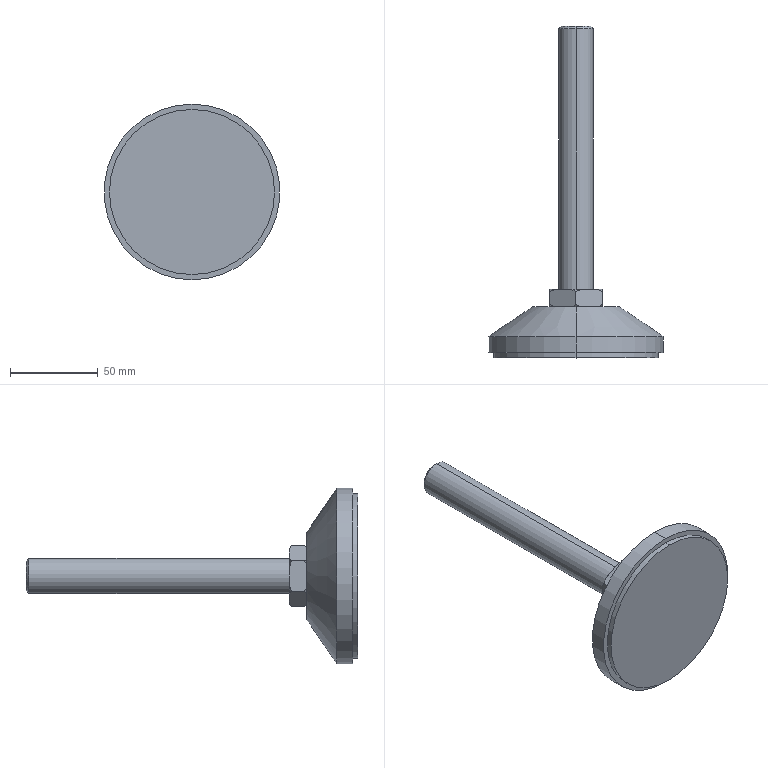Part | SolidWorks | features BaseBody 1 | 1 solid | 35 faces | box 100 x 189 x 100 mm | volume 224213 mm3 | spline 14 | plane 11 | cylinder 6 | cone 4 | commonest cylinder face diameters 20 x2 94 x2 100 x2